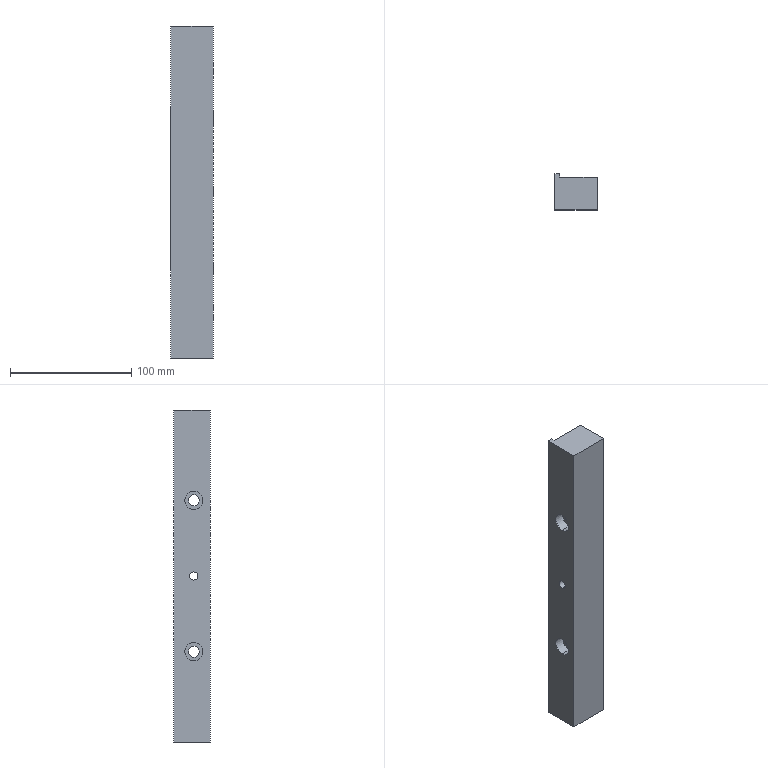Part | STEP file | LM-05-1243_default | 1 solid | 28 faces | box 35 x 30 x 274 mm | volume 250341 mm3 | cylinder 14 | plane 10 | cone 4 | commonest cylinder face diameters 9 x4 12 x4 15 x4 6.8 x2